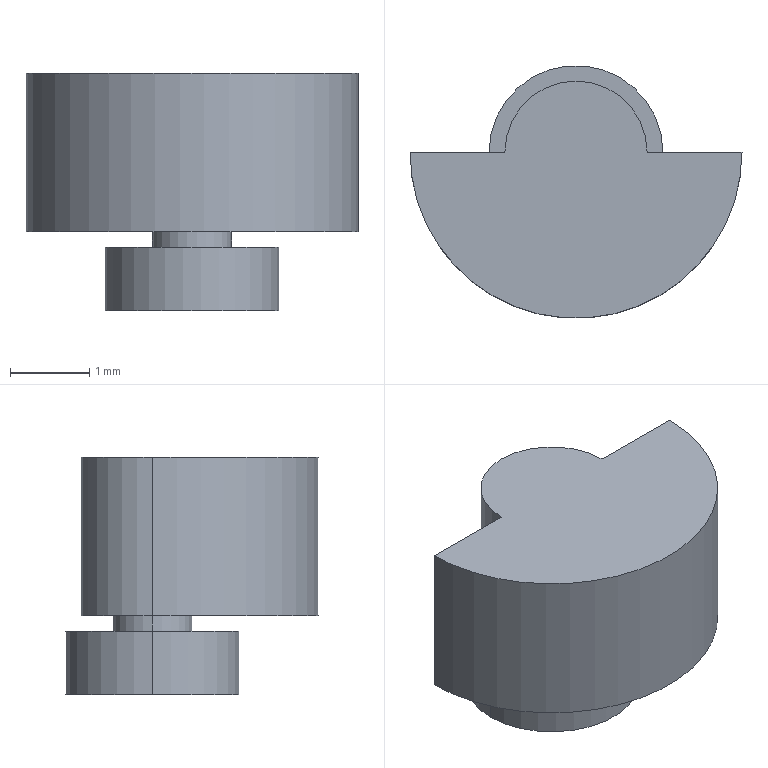Part | Creo | 1 solid | 12 faces | box 4.2 x 3.2 x 3 mm | volume 19.597 mm3 | plane 6 | cylinder 6 | commonest cylinder face diameters 1 x2 2.2 x2 1.8 x1 4.2 x1
STEP:
#1=CARTESIAN_POINT('',(0.,0.,0.));
#2=DIRECTION('',(0.,0.,1.));
#3=DIRECTION('',(1.,0.,0.));
#4=AXIS2_PLACEMENT_3D('',#1,#2,#3);
#5=CARTESIAN_POINT('',(3.6,2.3,8.8));
#6=VERTEX_POINT('',#5);
#7=CARTESIAN_POINT('',(1.4,2.3,8.8));
#8=VERTEX_POINT('',#7);
#9=CARTESIAN_POINT('',(2.5,2.3,8.8));
#10=DIRECTION('',(0.,0.,1.));
#11=DIRECTION('',(1.,0.,0.));
#12=AXIS2_PLACEMENT_3D('',#9,#10,#11);
#13=CIRCLE('',#12,1.1);
#14=EDGE_CURVE('',#6,#8,#13,.T.);
#15=ORIENTED_EDGE('',*,*,#14,.T.);
#16=CARTESIAN_POINT('',(2.5,2.3,8.8));
#17=DIRECTION('',(0.,0.,1.));
#18=DIRECTION('',(-1.,0.,0.));
#19=AXIS2_PLACEMENT_3D('',#16,#17,#18);
#20=CIRCLE('',#19,1.1);
#21=EDGE_CURVE('',#8,#6,#20,.T.);
#22=ORIENTED_EDGE('',*,*,#21,.T.);
#23=EDGE_LOOP('',(#15,#22));
#24=FACE_OUTER_BOUND('',#23,.F.);
#25=CARTESIAN_POINT('',(0.,0.,8.8));
#26=DIRECTION('',(0.,0.,1.));
#27=DIRECTION('',(1.,0.,0.));
#28=AXIS2_PLACEMENT_3D('',#25,#26,#27);
#29=PLANE('',#28);
#30=ADVANCED_FACE('',(#24),#29,.F.);
#31=ORIENTED_EDGE('',*,*,#14,.F.);
#32=CARTESIAN_POINT('',(3.6,2.3,9.6));
#33=VERTEX_POINT('',#32);
#34=CARTESIAN_POINT('',(3.6,2.3,9.6));
#35=DIRECTION('',(0.,0.,-1.));
#36=VECTOR('',#35,0.8);
#37=LINE('',#34,#36);
#38=EDGE_CURVE('',#33,#6,#37,.T.);
#39=ORIENTED_EDGE('',*,*,#38,.F.);
#40=CARTESIAN_POINT('',(1.4,2.3,9.6));
#41=VERTEX_POINT('',#40);
#42=CARTESIAN_POINT('',(2.5,2.3,9.6));
#43=DIRECTION('',(0.,0.,-1.));
#44=DIRECTION('',(-1.,0.,0.));
#45=AXIS2_PLACEMENT_3D('',#42,#43,#44);
#46=CIRCLE('',#45,1.1);
#47=EDGE_CURVE('',#41,#33,#46,.T.);
#48=ORIENTED_EDGE('',*,*,#47,.F.);
#49=CARTESIAN_POINT('',(1.4,2.3,9.6));
#50=DIRECTION('',(0.,0.,-1.));
#51=VECTOR('',#50,0.8);
#52=LINE('',#49,#51);
#53=EDGE_CURVE('',#41,#8,#52,.T.);
#54=ORIENTED_EDGE('',*,*,#53,.T.);
#55=EDGE_LOOP('',(#31,#39,#48,#54));
#56=FACE_OUTER_BOUND('',#55,.F.);
#57=CARTESIAN_POINT('',(2.5,2.3,8.8));
#58=DIRECTION('',(0.,0.,1.));
#59=DIRECTION('',(1.,0.,0.));
#60=AXIS2_PLACEMENT_3D('',#57,#58,#59);
#61=CYLINDRICAL_SURFACE('',#60,1.1);
#62=ADVANCED_FACE('',(#56),#61,.T.);
#63=ORIENTED_EDGE('',*,*,#21,.F.);
#64=ORIENTED_EDGE('',*,*,#53,.F.);
#65=CARTESIAN_POINT('',(2.5,2.3,9.6));
#66=DIRECTION('',(0.,0.,-1.));
#67=DIRECTION('',(1.,0.,0.));
#68=AXIS2_PLACEMENT_3D('',#65,#66,#67);
#69=CIRCLE('',#68,1.1);
#70=EDGE_CURVE('',#33,#41,#69,.T.);
#71=ORIENTED_EDGE('',*,*,#70,.F.);
#72=ORIENTED_EDGE('',*,*,#38,.T.);
#73=EDGE_LOOP('',(#63,#64,#71,#72));
#74=FACE_OUTER_BOUND('',#73,.F.);
#75=CARTESIAN_POINT('',(2.5,2.3,8.8));
#76=DIRECTION('',(0.,0.,1.));
#77=DIRECTION('',(1.,0.,0.));
#78=AXIS2_PLACEMENT_3D('',#75,#76,#77);
#79=CYLINDRICAL_SURFACE('',#78,1.1);
#80=ADVANCED_FACE('',(#74),#79,.T.);
#81=ORIENTED_EDGE('',*,*,#47,.T.);
#82=ORIENTED_EDGE('',*,*,#70,.T.);
#83=EDGE_LOOP('',(#81,#82));
#84=FACE_OUTER_BOUND('',#83,.F.);
#85=CARTESIAN_POINT('',(2.,2.3,9.6));
#86=VERTEX_POINT('',#85);
#87=CARTESIAN_POINT('',(3.,2.3,9.6));
#88=VERTEX_POINT('',#87);
#89=CARTESIAN_POINT('',(2.5,2.3,9.6));
#90=DIRECTION('',(0.,0.,1.));
#91=DIRECTION('',(-1.,0.,0.));
#92=AXIS2_PLACEMENT_3D('',#89,#90,#91);
#93=CIRCLE('',#92,0.5);
#94=EDGE_CURVE('',#86,#88,#93,.T.);
#95=ORIENTED_EDGE('',*,*,#94,.T.);
#96=CARTESIAN_POINT('',(2.5,2.3,9.6));
#97=DIRECTION('',(0.,0.,1.));
#98=DIRECTION('',(1.,0.,0.));
#99=AXIS2_PLACEMENT_3D('',#96,#97,#98);
#100=CIRCLE('',#99,0.5);
#101=EDGE_CURVE('',#88,#86,#100,.T.);
#102=ORIENTED_EDGE('',*,*,#101,.T.);
#103=EDGE_LOOP('',(#95,#102));
#104=FACE_BOUND('',#103,.F.);
#105=CARTESIAN_POINT('',(0.,0.,9.6));
#106=DIRECTION('',(0.,0.,-1.));
#107=DIRECTION('',(-1.,0.,0.));
#108=AXIS2_PLACEMENT_3D('',#105,#106,#107);
#109=PLANE('',#108);
#110=ADVANCED_FACE('',(#84,#104),#109,.F.);
#111=CARTESIAN_POINT('',(3.,2.3,9.8));
#112=VERTEX_POINT('',#111);
#113=CARTESIAN_POINT('',(2.,2.3,9.8));
#114=VERTEX_POINT('',#113);
#115=CARTESIAN_POINT('',(2.5,2.3,9.8));
#116=DIRECTION('',(0.,0.,-1.));
#117=DIRECTION('',(1.,0.,0.));
#118=AXIS2_PLACEMENT_3D('',#115,#116,#117);
#119=CIRCLE('',#118,0.5);
#120=EDGE_CURVE('',#112,#114,#119,.T.);
#121=ORIENTED_EDGE('',*,*,#120,.F.);
#122=CARTESIAN_POINT('',(3.,2.3,9.6));
#123=DIRECTION('',(0.,0.,1.));
#124=VECTOR('',#123,0.2);
#125=LINE('',#122,#124);
#126=EDGE_CURVE('',#88,#112,#125,.T.);
#127=ORIENTED_EDGE('',*,*,#126,.F.);
#128=ORIENTED_EDGE('',*,*,#94,.F.);
#129=CARTESIAN_POINT('',(2.,2.3,9.6));
#130=DIRECTION('',(0.,0.,1.));
#131=VECTOR('',#130,0.2);
#132=LINE('',#129,#131);
#133=EDGE_CURVE('',#86,#114,#132,.T.);
#134=ORIENTED_EDGE('',*,*,#133,.T.);
#135=EDGE_LOOP('',(#121,#127,#128,#134));
#136=FACE_OUTER_BOUND('',#135,.F.);
#137=CARTESIAN_POINT('',(2.5,2.3,9.8));
#138=DIRECTION('',(0.,0.,-1.));
#139=DIRECTION('',(-1.,0.,0.));
#140=AXIS2_PLACEMENT_3D('',#137,#138,#139);
#141=CYLINDRICAL_SURFACE('',#140,0.5);
#142=ADVANCED_FACE('',(#136),#141,.T.);
#143=CARTESIAN_POINT('',(3.4,2.3,9.8));
#144=VERTEX_POINT('',#143);
#145=CARTESIAN_POINT('',(4.6,2.3,9.8));
#146=VERTEX_POINT('',#145);
#147=CARTESIAN_POINT('',(3.4,2.3,9.8));
#148=DIRECTION('',(1.,0.,0.));
#149=VECTOR('',#148,1.2);
#150=LINE('',#147,#149);
#151=EDGE_CURVE('',#144,#146,#150,.T.);
#152=ORIENTED_EDGE('',*,*,#151,.F.);
#153=CARTESIAN_POINT('',(1.6,2.3,9.8));
#154=VERTEX_POINT('',#153);
#155=CARTESIAN_POINT('',(2.5,2.3,9.8));
#156=DIRECTION('',(0.,0.,1.));
#157=DIRECTION('',(1.,0.,0.));
#158=AXIS2_PLACEMENT_3D('',#155,#156,#157);
#159=CIRCLE('',#158,0.9);
#160=EDGE_CURVE('',#144,#154,#159,.T.);
#161=ORIENTED_EDGE('',*,*,#160,.T.);
#162=CARTESIAN_POINT('',(0.4,2.3,9.8));
#163=VERTEX_POINT('',#162);
#164=CARTESIAN_POINT('',(0.4,2.3,9.8));
#165=DIRECTION('',(1.,0.,0.));
#166=VECTOR('',#165,1.2);
#167=LINE('',#164,#166);
#168=EDGE_CURVE('',#163,#154,#167,.T.);
#169=ORIENTED_EDGE('',*,*,#168,.F.);
#170=CARTESIAN_POINT('',(2.5,2.3,9.8));
#171=DIRECTION('',(0.,0.,1.));
#172=DIRECTION('',(-1.,0.,0.));
#173=AXIS2_PLACEMENT_3D('',#170,#171,#172);
#174=CIRCLE('',#173,2.1);
#175=EDGE_CURVE('',#163,#146,#174,.T.);
#176=ORIENTED_EDGE('',*,*,#175,.T.);
#177=EDGE_LOOP('',(#152,#161,#169,#176));
#178=FACE_OUTER_BOUND('',#177,.F.);
#179=ORIENTED_EDGE('',*,*,#120,.T.);
#180=CARTESIAN_POINT('',(2.5,2.3,9.8));
#181=DIRECTION('',(0.,0.,-1.));
#182=DIRECTION('',(-1.,0.,0.));
#183=AXIS2_PLACEMENT_3D('',#180,#181,#182);
#184=CIRCLE('',#183,0.5);
#185=EDGE_CURVE('',#114,#112,#184,.T.);
#186=ORIENTED_EDGE('',*,*,#185,.T.);
#187=EDGE_LOOP('',(#179,#186));
#188=FACE_BOUND('',#187,.F.);
#189=CARTESIAN_POINT('',(0.,0.,9.8));
#190=DIRECTION('',(0.,0.,1.));
#191=DIRECTION('',(1.,0.,0.));
#192=AXIS2_PLACEMENT_3D('',#189,#190,#191);
#193=PLANE('',#192);
#194=ADVANCED_FACE('',(#178,#188),#193,.F.);
#195=ORIENTED_EDGE('',*,*,#151,.T.);
#196=CARTESIAN_POINT('',(4.6,2.3,11.8));
#197=VERTEX_POINT('',#196);
#198=CARTESIAN_POINT('',(4.6,2.3,11.8));
#199=DIRECTION('',(0.,0.,-1.));
#200=VECTOR('',#199,2.);
#201=LINE('',#198,#200);
#202=EDGE_CURVE('',#197,#146,#201,.T.);
#203=ORIENTED_EDGE('',*,*,#202,.F.);
#204=CARTESIAN_POINT('',(3.4,2.3,11.8));
#205=VERTEX_POINT('',#204);
#206=CARTESIAN_POINT('',(3.4,2.3,11.8));
#207=DIRECTION('',(1.,0.,0.));
#208=VECTOR('',#207,1.2);
#209=LINE('',#206,#208);
#210=EDGE_CURVE('',#205,#197,#209,.T.);
#211=ORIENTED_EDGE('',*,*,#210,.F.);
#212=CARTESIAN_POINT('',(3.4,2.3,9.8));
#213=DIRECTION('',(0.,0.,1.));
#214=VECTOR('',#213,2.);
#215=LINE('',#212,#214);
#216=EDGE_CURVE('',#144,#205,#215,.T.);
#217=ORIENTED_EDGE('',*,*,#216,.F.);
#218=EDGE_LOOP('',(#195,#203,#211,#217));
#219=FACE_OUTER_BOUND('',#218,.F.);
#220=CARTESIAN_POINT('',(3.4,2.3,11.8));
#221=DIRECTION('',(0.,-1.,0.));
#222=DIRECTION('',(1.,0.,0.));
#223=AXIS2_PLACEMENT_3D('',#220,#221,#222);
#224=PLANE('',#223);
#225=ADVANCED_FACE('',(#219),#224,.F.);
#226=CARTESIAN_POINT('',(0.4,2.3,11.8));
#227=VERTEX_POINT('',#226);
#228=CARTESIAN_POINT('',(0.4,2.3,9.8));
#229=DIRECTION('',(0.,0.,1.));
#230=VECTOR('',#229,2.);
#231=LINE('',#228,#230);
#232=EDGE_CURVE('',#163,#227,#231,.T.);
#233=ORIENTED_EDGE('',*,*,#232,.T.);
#234=CARTESIAN_POINT('',(2.5,2.3,11.8));
#235=DIRECTION('',(0.,0.,-1.));
#236=DIRECTION('',(1.,0.,0.));
#237=AXIS2_PLACEMENT_3D('',#234,#235,#236);
#238=CIRCLE('',#237,2.1);
#239=EDGE_CURVE('',#197,#227,#238,.T.);
#240=ORIENTED_EDGE('',*,*,#239,.F.);
#241=ORIENTED_EDGE('',*,*,#202,.T.);
#242=ORIENTED_EDGE('',*,*,#175,.F.);
#243=EDGE_LOOP('',(#233,#240,#241,#242));
#244=FACE_OUTER_BOUND('',#243,.F.);
#245=CARTESIAN_POINT('',(2.5,2.3,11.8));
#246=DIRECTION('',(0.,0.,1.));
#247=DIRECTION('',(1.,0.,0.));
#248=AXIS2_PLACEMENT_3D('',#245,#246,#247);
#249=CYLINDRICAL_SURFACE('',#248,2.1);
#250=ADVANCED_FACE('',(#244),#249,.T.);
#251=ORIENTED_EDGE('',*,*,#168,.T.);
#252=CARTESIAN_POINT('',(1.6,2.3,11.8));
#253=VERTEX_POINT('',#252);
#254=CARTESIAN_POINT('',(1.6,2.3,11.8));
#255=DIRECTION('',(0.,0.,-1.));
#256=VECTOR('',#255,2.);
#257=LINE('',#254,#256);
#258=EDGE_CURVE('',#253,#154,#257,.T.);
#259=ORIENTED_EDGE('',*,*,#258,.F.);
#260=CARTESIAN_POINT('',(1.6,2.3,11.8));
#261=DIRECTION('',(-1.,0.,0.));
#262=VECTOR('',#261,1.2);
#263=LINE('',#260,#262);
#264=EDGE_CURVE('',#253,#227,#263,.T.);
#265=ORIENTED_EDGE('',*,*,#264,.T.);
#266=ORIENTED_EDGE('',*,*,#232,.F.);
#267=EDGE_LOOP('',(#251,#259,#265,#266));
#268=FACE_OUTER_BOUND('',#267,.F.);
#269=CARTESIAN_POINT('',(0.4,2.3,11.8));
#270=DIRECTION('',(0.,-1.,0.));
#271=DIRECTION('',(1.,0.,0.));
#272=AXIS2_PLACEMENT_3D('',#269,#270,#271);
#273=PLANE('',#272);
#274=ADVANCED_FACE('',(#268),#273,.F.);
#275=ORIENTED_EDGE('',*,*,#160,.F.);
#276=ORIENTED_EDGE('',*,*,#216,.T.);
#277=CARTESIAN_POINT('',(2.5,2.3,11.8));
#278=DIRECTION('',(0.,0.,-1.));
#279=DIRECTION('',(-1.,0.,0.));
#280=AXIS2_PLACEMENT_3D('',#277,#278,#279);
#281=CIRCLE('',#280,0.9);
#282=EDGE_CURVE('',#253,#205,#281,.T.);
#283=ORIENTED_EDGE('',*,*,#282,.F.);
#284=ORIENTED_EDGE('',*,*,#258,.T.);
#285=EDGE_LOOP('',(#275,#276,#283,#284));
#286=FACE_OUTER_BOUND('',#285,.F.);
#287=CARTESIAN_POINT('',(2.5,2.3,11.8));
#288=DIRECTION('',(0.,0.,1.));
#289=DIRECTION('',(1.,0.,0.));
#290=AXIS2_PLACEMENT_3D('',#287,#288,#289);
#291=CYLINDRICAL_SURFACE('',#290,0.9);
#292=ADVANCED_FACE('',(#286),#291,.T.);
#293=ORIENTED_EDGE('',*,*,#264,.F.);
#294=ORIENTED_EDGE('',*,*,#282,.T.);
#295=ORIENTED_EDGE('',*,*,#210,.T.);
#296=ORIENTED_EDGE('',*,*,#239,.T.);
#297=EDGE_LOOP('',(#293,#294,#295,#296));
#298=FACE_OUTER_BOUND('',#297,.F.);
#299=CARTESIAN_POINT('',(0.,0.,11.8));
#300=DIRECTION('',(0.,0.,1.));
#301=DIRECTION('',(1.,0.,0.));
#302=AXIS2_PLACEMENT_3D('',#299,#300,#301);
#303=PLANE('',#302);
#304=ADVANCED_FACE('',(#298),#303,.T.);
#305=ORIENTED_EDGE('',*,*,#185,.F.);
#306=ORIENTED_EDGE('',*,*,#133,.F.);
#307=ORIENTED_EDGE('',*,*,#101,.F.);
#308=ORIENTED_EDGE('',*,*,#126,.T.);
#309=EDGE_LOOP('',(#305,#306,#307,#308));
#310=FACE_OUTER_BOUND('',#309,.F.);
#311=CARTESIAN_POINT('',(2.5,2.3,9.8));
#312=DIRECTION('',(0.,0.,-1.));
#313=DIRECTION('',(-1.,0.,0.));
#314=AXIS2_PLACEMENT_3D('',#311,#312,#313);
#315=CYLINDRICAL_SURFACE('',#314,0.5);
#316=ADVANCED_FACE('',(#310),#315,.T.);
#317=CLOSED_SHELL('',(#30,#62,#80,#110,#142,#194,#225,#250,#274,#292,#304,#316));
#318=MANIFOLD_SOLID_BREP('',#317);
#319=(LENGTH_UNIT()NAMED_UNIT(*)SI_UNIT(.MILLI.,.METRE.));
#320=UNCERTAINTY_MEASURE_WITH_UNIT(LENGTH_MEASURE(0.0006073),#319,'','');
#321=(NAMED_UNIT(*)PLANE_ANGLE_UNIT()SI_UNIT($,.RADIAN.));
#322=PLANE_ANGLE_MEASURE_WITH_UNIT(PLANE_ANGLE_MEASURE(0.01745),#321);
#323=(CONVERSION_BASED_UNIT('DEGREE',#322)NAMED_UNIT(*)PLANE_ANGLE_UNIT());
#324=(NAMED_UNIT(*)SI_UNIT($,.STERADIAN.)SOLID_ANGLE_UNIT());
#325=(GEOMETRIC_REPRESENTATION_CONTEXT(3)GLOBAL_UNCERTAINTY_ASSIGNED_CONTEXT((#320))GLOBAL_UNIT_ASSIGNED_CONTEXT((#319,#323,#324))REPRESENTATION_CONTEXT('',''));
#326=ADVANCED_BREP_SHAPE_REPRESENTATION('',(#4,#318),#325);